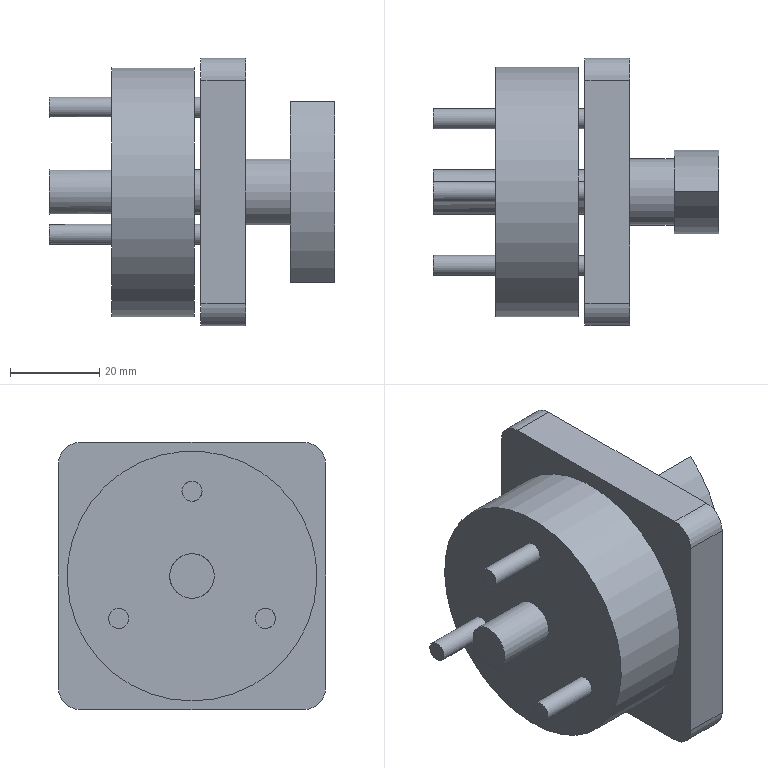Part | STEP file | 冲床-300配套压波_id418_x_t | 1 solid | 30 faces | box 64 x 60 x 60 mm | volume 90346 mm3 | cylinder 16 | plane 14 | commonest cylinder face diameters 4.5 x6 10 x6 53.607 x2 15 x1 56 x1
STEP:
#1=CARTESIAN_POINT('',(1921.2,181.454,-152.25));
#2=VERTEX_POINT('',#1);
#3=CARTESIAN_POINT('',(1921.2,181.454,-154.5));
#4=DIRECTION('',(1.,0.,0.));
#5=DIRECTION('',(0.,0.,1.));
#6=AXIS2_PLACEMENT_3D('',#3,#4,#5);
#7=CIRCLE('',#6,2.25);
#8=EDGE_CURVE('',#2,#2,#7,.T.);
#9=ORIENTED_EDGE('',*,*,#8,.F.);
#10=EDGE_LOOP('',(#9));
#11=FACE_BOUND('',#10,.T.);
#12=CARTESIAN_POINT('',(1919.7,181.454,-156.75));
#13=VERTEX_POINT('',#12);
#14=CARTESIAN_POINT('',(1919.7,181.454,-154.5));
#15=DIRECTION('',(1.,0.,0.));
#16=DIRECTION('',(0.,0.,-1.));
#17=AXIS2_PLACEMENT_3D('',#14,#15,#16);
#18=CIRCLE('',#17,2.25);
#19=EDGE_CURVE('',#13,#13,#18,.T.);
#20=ORIENTED_EDGE('',*,*,#19,.T.);
#21=EDGE_LOOP('',(#20));
#22=FACE_BOUND('',#21,.T.);
#23=CARTESIAN_POINT('',(1887.2,181.454,-154.5));
#24=DIRECTION('',(1.,0.,0.));
#25=DIRECTION('',(0.,0.,1.));
#26=AXIS2_PLACEMENT_3D('',#23,#24,#25);
#27=CYLINDRICAL_SURFACE('',#26,2.25);
#28=ADVANCED_FACE('',(#11,#22),#27,.T.);
#29=CARTESIAN_POINT('',(1921.2,165.,-123.75));
#30=VERTEX_POINT('',#29);
#31=CARTESIAN_POINT('',(1921.2,165.,-126.));
#32=DIRECTION('',(1.,0.,0.));
#33=DIRECTION('',(0.,0.,1.));
#34=AXIS2_PLACEMENT_3D('',#31,#32,#33);
#35=CIRCLE('',#34,2.25);
#36=EDGE_CURVE('',#30,#30,#35,.T.);
#37=ORIENTED_EDGE('',*,*,#36,.F.);
#38=EDGE_LOOP('',(#37));
#39=FACE_BOUND('',#38,.T.);
#40=CARTESIAN_POINT('',(1919.7,165.,-128.25));
#41=VERTEX_POINT('',#40);
#42=CARTESIAN_POINT('',(1919.7,165.,-126.));
#43=DIRECTION('',(1.,0.,0.));
#44=DIRECTION('',(0.,0.,-1.));
#45=AXIS2_PLACEMENT_3D('',#42,#43,#44);
#46=CIRCLE('',#45,2.25);
#47=EDGE_CURVE('',#41,#41,#46,.T.);
#48=ORIENTED_EDGE('',*,*,#47,.T.);
#49=EDGE_LOOP('',(#48));
#50=FACE_BOUND('',#49,.T.);
#51=CARTESIAN_POINT('',(1887.2,165.,-126.));
#52=DIRECTION('',(1.,0.,0.));
#53=DIRECTION('',(0.,0.,1.));
#54=AXIS2_PLACEMENT_3D('',#51,#52,#53);
#55=CYLINDRICAL_SURFACE('',#54,2.25);
#56=ADVANCED_FACE('',(#39,#50),#55,.T.);
#57=CARTESIAN_POINT('',(1921.2,165.,-140.));
#58=VERTEX_POINT('',#57);
#59=CARTESIAN_POINT('',(1921.2,165.,-145.));
#60=DIRECTION('',(1.,0.,0.));
#61=DIRECTION('',(0.,0.,1.));
#62=AXIS2_PLACEMENT_3D('',#59,#60,#61);
#63=CIRCLE('',#62,5.);
#64=EDGE_CURVE('',#58,#58,#63,.T.);
#65=ORIENTED_EDGE('',*,*,#64,.F.);
#66=EDGE_LOOP('',(#65));
#67=FACE_BOUND('',#66,.T.);
#68=CARTESIAN_POINT('',(1919.7,165.,-150.));
#69=VERTEX_POINT('',#68);
#70=CARTESIAN_POINT('',(1919.7,165.,-145.));
#71=DIRECTION('',(1.,0.,0.));
#72=DIRECTION('',(0.,0.,-1.));
#73=AXIS2_PLACEMENT_3D('',#70,#71,#72);
#74=CIRCLE('',#73,5.);
#75=EDGE_CURVE('',#69,#69,#74,.T.);
#76=ORIENTED_EDGE('',*,*,#75,.T.);
#77=EDGE_LOOP('',(#76));
#78=FACE_BOUND('',#77,.T.);
#79=CARTESIAN_POINT('',(1887.2,165.,-145.));
#80=DIRECTION('',(1.,0.,0.));
#81=DIRECTION('',(0.,0.,1.));
#82=AXIS2_PLACEMENT_3D('',#79,#80,#81);
#83=CYLINDRICAL_SURFACE('',#82,5.);
#84=ADVANCED_FACE('',(#67,#78),#83,.T.);
#85=CARTESIAN_POINT('',(1921.2,148.546,-152.25));
#86=VERTEX_POINT('',#85);
#87=CARTESIAN_POINT('',(1921.2,148.546,-154.5));
#88=DIRECTION('',(1.,0.,0.));
#89=DIRECTION('',(0.,0.,1.));
#90=AXIS2_PLACEMENT_3D('',#87,#88,#89);
#91=CIRCLE('',#90,2.25);
#92=EDGE_CURVE('',#86,#86,#91,.T.);
#93=ORIENTED_EDGE('',*,*,#92,.F.);
#94=EDGE_LOOP('',(#93));
#95=FACE_BOUND('',#94,.T.);
#96=CARTESIAN_POINT('',(1919.7,148.546,-156.75));
#97=VERTEX_POINT('',#96);
#98=CARTESIAN_POINT('',(1919.7,148.546,-154.5));
#99=DIRECTION('',(1.,0.,0.));
#100=DIRECTION('',(0.,0.,-1.));
#101=AXIS2_PLACEMENT_3D('',#98,#99,#100);
#102=CIRCLE('',#101,2.25);
#103=EDGE_CURVE('',#97,#97,#102,.T.);
#104=ORIENTED_EDGE('',*,*,#103,.T.);
#105=EDGE_LOOP('',(#104));
#106=FACE_BOUND('',#105,.T.);
#107=CARTESIAN_POINT('',(1887.2,148.546,-154.5));
#108=DIRECTION('',(1.,0.,0.));
#109=DIRECTION('',(0.,0.,1.));
#110=AXIS2_PLACEMENT_3D('',#107,#108,#109);
#111=CYLINDRICAL_SURFACE('',#110,2.25);
#112=ADVANCED_FACE('',(#95,#106),#111,.T.);
#113=CARTESIAN_POINT('',(1931.2,135.,-120.));
#114=VERTEX_POINT('',#113);
#115=CARTESIAN_POINT('',(1931.2,135.,-170.));
#116=VERTEX_POINT('',#115);
#117=CARTESIAN_POINT('',(1931.2,135.,-175.));
#118=DIRECTION('',(0.,0.,-1.));
#119=VECTOR('',#118,1.);
#120=LINE('',#117,#119);
#121=EDGE_CURVE('',#114,#116,#120,.T.);
#122=ORIENTED_EDGE('',*,*,#121,.F.);
#123=CARTESIAN_POINT('',(1921.2,135.,-120.));
#124=VERTEX_POINT('',#123);
#125=CARTESIAN_POINT('',(1931.2,135.,-120.));
#126=DIRECTION('',(-1.,0.,0.));
#127=VECTOR('',#126,1.);
#128=LINE('',#125,#127);
#129=EDGE_CURVE('',#114,#124,#128,.T.);
#130=ORIENTED_EDGE('',*,*,#129,.T.);
#131=CARTESIAN_POINT('',(1921.2,135.,-170.));
#132=VERTEX_POINT('',#131);
#133=CARTESIAN_POINT('',(1921.2,135.,-175.));
#134=DIRECTION('',(0.,0.,-1.));
#135=VECTOR('',#134,1.);
#136=LINE('',#133,#135);
#137=EDGE_CURVE('',#124,#132,#136,.T.);
#138=ORIENTED_EDGE('',*,*,#137,.T.);
#139=CARTESIAN_POINT('',(1931.2,135.,-170.));
#140=DIRECTION('',(1.,0.,0.));
#141=VECTOR('',#140,1.);
#142=LINE('',#139,#141);
#143=EDGE_CURVE('',#132,#116,#142,.T.);
#144=ORIENTED_EDGE('',*,*,#143,.T.);
#145=EDGE_LOOP('',(#122,#130,#138,#144));
#146=FACE_OUTER_BOUND('',#145,.T.);
#147=CARTESIAN_POINT('',(1931.2,135.,-175.));
#148=DIRECTION('',(0.,1.,0.));
#149=DIRECTION('',(0.,0.,-1.));
#150=AXIS2_PLACEMENT_3D('',#147,#148,#149);
#151=PLANE('',#150);
#152=ADVANCED_FACE('',(#146),#151,.F.);
#153=CARTESIAN_POINT('',(1921.2,190.,-115.));
#154=VERTEX_POINT('',#153);
#155=CARTESIAN_POINT('',(1921.2,140.,-115.));
#156=VERTEX_POINT('',#155);
#157=CARTESIAN_POINT('',(1921.2,135.,-115.));
#158=DIRECTION('',(0.,-1.,0.));
#159=VECTOR('',#158,1.);
#160=LINE('',#157,#159);
#161=EDGE_CURVE('',#154,#156,#160,.T.);
#162=ORIENTED_EDGE('',*,*,#161,.T.);
#163=CARTESIAN_POINT('',(1931.2,140.,-115.));
#164=VERTEX_POINT('',#163);
#165=CARTESIAN_POINT('',(1931.2,140.,-115.));
#166=DIRECTION('',(1.,0.,0.));
#167=VECTOR('',#166,1.);
#168=LINE('',#165,#167);
#169=EDGE_CURVE('',#156,#164,#168,.T.);
#170=ORIENTED_EDGE('',*,*,#169,.T.);
#171=CARTESIAN_POINT('',(1931.2,190.,-115.));
#172=VERTEX_POINT('',#171);
#173=CARTESIAN_POINT('',(1931.2,135.,-115.));
#174=DIRECTION('',(0.,-1.,0.));
#175=VECTOR('',#174,1.);
#176=LINE('',#173,#175);
#177=EDGE_CURVE('',#172,#164,#176,.T.);
#178=ORIENTED_EDGE('',*,*,#177,.F.);
#179=CARTESIAN_POINT('',(1931.2,190.,-115.));
#180=DIRECTION('',(-1.,0.,0.));
#181=VECTOR('',#180,1.);
#182=LINE('',#179,#181);
#183=EDGE_CURVE('',#172,#154,#182,.T.);
#184=ORIENTED_EDGE('',*,*,#183,.T.);
#185=EDGE_LOOP('',(#162,#170,#178,#184));
#186=FACE_OUTER_BOUND('',#185,.T.);
#187=CARTESIAN_POINT('',(1931.2,135.,-115.));
#188=DIRECTION('',(0.,0.,-1.));
#189=DIRECTION('',(0.,-1.,0.));
#190=AXIS2_PLACEMENT_3D('',#187,#188,#189);
#191=PLANE('',#190);
#192=ADVANCED_FACE('',(#186),#191,.F.);
#193=CARTESIAN_POINT('',(1921.2,195.,-170.));
#194=VERTEX_POINT('',#193);
#195=CARTESIAN_POINT('',(1921.2,195.,-120.));
#196=VERTEX_POINT('',#195);
#197=CARTESIAN_POINT('',(1921.2,195.,-115.));
#198=DIRECTION('',(0.,0.,1.));
#199=VECTOR('',#198,1.);
#200=LINE('',#197,#199);
#201=EDGE_CURVE('',#194,#196,#200,.T.);
#202=ORIENTED_EDGE('',*,*,#201,.T.);
#203=CARTESIAN_POINT('',(1931.2,195.,-120.));
#204=VERTEX_POINT('',#203);
#205=CARTESIAN_POINT('',(1931.2,195.,-120.));
#206=DIRECTION('',(1.,0.,0.));
#207=VECTOR('',#206,1.);
#208=LINE('',#205,#207);
#209=EDGE_CURVE('',#196,#204,#208,.T.);
#210=ORIENTED_EDGE('',*,*,#209,.T.);
#211=CARTESIAN_POINT('',(1931.2,195.,-170.));
#212=VERTEX_POINT('',#211);
#213=CARTESIAN_POINT('',(1931.2,195.,-115.));
#214=DIRECTION('',(0.,0.,1.));
#215=VECTOR('',#214,1.);
#216=LINE('',#213,#215);
#217=EDGE_CURVE('',#212,#204,#216,.T.);
#218=ORIENTED_EDGE('',*,*,#217,.F.);
#219=CARTESIAN_POINT('',(1931.2,195.,-170.));
#220=DIRECTION('',(-1.,0.,0.));
#221=VECTOR('',#220,1.);
#222=LINE('',#219,#221);
#223=EDGE_CURVE('',#212,#194,#222,.T.);
#224=ORIENTED_EDGE('',*,*,#223,.T.);
#225=EDGE_LOOP('',(#202,#210,#218,#224));
#226=FACE_OUTER_BOUND('',#225,.T.);
#227=CARTESIAN_POINT('',(1931.2,195.,-115.));
#228=DIRECTION('',(0.,-1.,0.));
#229=DIRECTION('',(0.,0.,1.));
#230=AXIS2_PLACEMENT_3D('',#227,#228,#229);
#231=PLANE('',#230);
#232=ADVANCED_FACE('',(#226),#231,.F.);
#233=CARTESIAN_POINT('',(1931.2,140.,-175.));
#234=VERTEX_POINT('',#233);
#235=CARTESIAN_POINT('',(1931.2,190.,-175.));
#236=VERTEX_POINT('',#235);
#237=CARTESIAN_POINT('',(1931.2,195.,-175.));
#238=DIRECTION('',(0.,1.,0.));
#239=VECTOR('',#238,1.);
#240=LINE('',#237,#239);
#241=EDGE_CURVE('',#234,#236,#240,.T.);
#242=ORIENTED_EDGE('',*,*,#241,.F.);
#243=CARTESIAN_POINT('',(1921.2,140.,-175.));
#244=VERTEX_POINT('',#243);
#245=CARTESIAN_POINT('',(1931.2,140.,-175.));
#246=DIRECTION('',(-1.,0.,0.));
#247=VECTOR('',#246,1.);
#248=LINE('',#245,#247);
#249=EDGE_CURVE('',#234,#244,#248,.T.);
#250=ORIENTED_EDGE('',*,*,#249,.T.);
#251=CARTESIAN_POINT('',(1921.2,190.,-175.));
#252=VERTEX_POINT('',#251);
#253=CARTESIAN_POINT('',(1921.2,195.,-175.));
#254=DIRECTION('',(0.,1.,0.));
#255=VECTOR('',#254,1.);
#256=LINE('',#253,#255);
#257=EDGE_CURVE('',#244,#252,#256,.T.);
#258=ORIENTED_EDGE('',*,*,#257,.T.);
#259=CARTESIAN_POINT('',(1931.2,190.,-175.));
#260=DIRECTION('',(1.,0.,0.));
#261=VECTOR('',#260,1.);
#262=LINE('',#259,#261);
#263=EDGE_CURVE('',#252,#236,#262,.T.);
#264=ORIENTED_EDGE('',*,*,#263,.T.);
#265=EDGE_LOOP('',(#242,#250,#258,#264));
#266=FACE_OUTER_BOUND('',#265,.T.);
#267=CARTESIAN_POINT('',(1931.2,195.,-175.));
#268=DIRECTION('',(0.,0.,1.));
#269=DIRECTION('',(0.,1.,0.));
#270=AXIS2_PLACEMENT_3D('',#267,#268,#269);
#271=PLANE('',#270);
#272=ADVANCED_FACE('',(#266),#271,.F.);
#273=CARTESIAN_POINT('',(1931.2,157.5,-145.));
#274=VERTEX_POINT('',#273);
#275=CARTESIAN_POINT('',(1931.2,165.,-145.));
#276=DIRECTION('',(-1.,0.,0.));
#277=DIRECTION('',(0.,-1.,0.));
#278=AXIS2_PLACEMENT_3D('',#275,#276,#277);
#279=CIRCLE('',#278,7.5);
#280=EDGE_CURVE('',#274,#274,#279,.T.);
#281=ORIENTED_EDGE('',*,*,#280,.T.);
#282=EDGE_LOOP('',(#281));
#283=FACE_BOUND('',#282,.T.);
#284=ORIENTED_EDGE('',*,*,#217,.T.);
#285=CARTESIAN_POINT('',(1931.2,190.,-120.));
#286=DIRECTION('',(1.,0.,0.));
#287=DIRECTION('',(0.,0.,1.));
#288=AXIS2_PLACEMENT_3D('',#285,#286,#287);
#289=CIRCLE('',#288,5.);
#290=EDGE_CURVE('',#204,#172,#289,.T.);
#291=ORIENTED_EDGE('',*,*,#290,.T.);
#292=ORIENTED_EDGE('',*,*,#177,.T.);
#293=CARTESIAN_POINT('',(1931.2,140.,-120.));
#294=DIRECTION('',(1.,0.,0.));
#295=DIRECTION('',(0.,0.,1.));
#296=AXIS2_PLACEMENT_3D('',#293,#294,#295);
#297=CIRCLE('',#296,5.);
#298=EDGE_CURVE('',#164,#114,#297,.T.);
#299=ORIENTED_EDGE('',*,*,#298,.T.);
#300=ORIENTED_EDGE('',*,*,#121,.T.);
#301=CARTESIAN_POINT('',(1931.2,140.,-170.));
#302=DIRECTION('',(1.,0.,0.));
#303=DIRECTION('',(0.,0.,1.));
#304=AXIS2_PLACEMENT_3D('',#301,#302,#303);
#305=CIRCLE('',#304,5.);
#306=EDGE_CURVE('',#116,#234,#305,.T.);
#307=ORIENTED_EDGE('',*,*,#306,.T.);
#308=ORIENTED_EDGE('',*,*,#241,.T.);
#309=CARTESIAN_POINT('',(1931.2,190.,-170.));
#310=DIRECTION('',(1.,0.,0.));
#311=DIRECTION('',(0.,0.,1.));
#312=AXIS2_PLACEMENT_3D('',#309,#310,#311);
#313=CIRCLE('',#312,5.);
#314=EDGE_CURVE('',#236,#212,#313,.T.);
#315=ORIENTED_EDGE('',*,*,#314,.T.);
#316=EDGE_LOOP('',(#284,#291,#292,#299,#300,#307,#308,#315));
#317=FACE_BOUND('',#316,.T.);
#318=CARTESIAN_POINT('',(1931.2,885.,370.));
#319=DIRECTION('',(1.,0.,0.));
#320=DIRECTION('',(0.,0.,1.));
#321=AXIS2_PLACEMENT_3D('',#318,#319,#320);
#322=PLANE('',#321);
#323=ADVANCED_FACE('',(#283,#317),#322,.T.);
#324=ORIENTED_EDGE('',*,*,#92,.T.);
#325=EDGE_LOOP('',(#324));
#326=FACE_BOUND('',#325,.T.);
#327=ORIENTED_EDGE('',*,*,#64,.T.);
#328=EDGE_LOOP('',(#327));
#329=FACE_BOUND('',#328,.T.);
#330=ORIENTED_EDGE('',*,*,#36,.T.);
#331=EDGE_LOOP('',(#330));
#332=FACE_BOUND('',#331,.T.);
#333=ORIENTED_EDGE('',*,*,#8,.T.);
#334=EDGE_LOOP('',(#333));
#335=FACE_BOUND('',#334,.T.);
#336=ORIENTED_EDGE('',*,*,#257,.F.);
#337=CARTESIAN_POINT('',(1921.2,140.,-170.));
#338=DIRECTION('',(-1.,0.,0.));
#339=DIRECTION('',(0.,0.,1.));
#340=AXIS2_PLACEMENT_3D('',#337,#338,#339);
#341=CIRCLE('',#340,5.);
#342=EDGE_CURVE('',#244,#132,#341,.T.);
#343=ORIENTED_EDGE('',*,*,#342,.T.);
#344=ORIENTED_EDGE('',*,*,#137,.F.);
#345=CARTESIAN_POINT('',(1921.2,140.,-120.));
#346=DIRECTION('',(-1.,0.,0.));
#347=DIRECTION('',(0.,0.,1.));
#348=AXIS2_PLACEMENT_3D('',#345,#346,#347);
#349=CIRCLE('',#348,5.);
#350=EDGE_CURVE('',#124,#156,#349,.T.);
#351=ORIENTED_EDGE('',*,*,#350,.T.);
#352=ORIENTED_EDGE('',*,*,#161,.F.);
#353=CARTESIAN_POINT('',(1921.2,190.,-120.));
#354=DIRECTION('',(-1.,0.,0.));
#355=DIRECTION('',(0.,0.,1.));
#356=AXIS2_PLACEMENT_3D('',#353,#354,#355);
#357=CIRCLE('',#356,5.);
#358=EDGE_CURVE('',#154,#196,#357,.T.);
#359=ORIENTED_EDGE('',*,*,#358,.T.);
#360=ORIENTED_EDGE('',*,*,#201,.F.);
#361=CARTESIAN_POINT('',(1921.2,190.,-170.));
#362=DIRECTION('',(-1.,0.,0.));
#363=DIRECTION('',(0.,0.,1.));
#364=AXIS2_PLACEMENT_3D('',#361,#362,#363);
#365=CIRCLE('',#364,5.);
#366=EDGE_CURVE('',#194,#252,#365,.T.);
#367=ORIENTED_EDGE('',*,*,#366,.T.);
#368=EDGE_LOOP('',(#336,#343,#344,#351,#352,#359,#360,#367));
#369=FACE_BOUND('',#368,.T.);
#370=CARTESIAN_POINT('',(1921.2,885.,370.));
#371=DIRECTION('',(1.,0.,0.));
#372=DIRECTION('',(0.,0.,1.));
#373=AXIS2_PLACEMENT_3D('',#370,#371,#372);
#374=PLANE('',#373);
#375=ADVANCED_FACE('',(#326,#329,#332,#335,#369),#374,.F.);
#376=CARTESIAN_POINT('',(1941.2,157.5,-145.));
#377=VERTEX_POINT('',#376);
#378=CARTESIAN_POINT('',(1941.2,165.,-145.));
#379=DIRECTION('',(-1.,0.,0.));
#380=DIRECTION('',(0.,-1.,0.));
#381=AXIS2_PLACEMENT_3D('',#378,#379,#380);
#382=CIRCLE('',#381,7.5);
#383=EDGE_CURVE('',#377,#377,#382,.T.);
#384=ORIENTED_EDGE('',*,*,#383,.T.);
#385=EDGE_LOOP('',(#384));
#386=FACE_BOUND('',#385,.T.);
#387=ORIENTED_EDGE('',*,*,#280,.F.);
#388=EDGE_LOOP('',(#387));
#389=FACE_BOUND('',#388,.T.);
#390=CARTESIAN_POINT('',(1941.2,165.,-145.));
#391=DIRECTION('',(-1.,0.,0.));
#392=DIRECTION('',(0.,0.,-1.));
#393=AXIS2_PLACEMENT_3D('',#390,#391,#392);
#394=CYLINDRICAL_SURFACE('',#393,7.5);
#395=ADVANCED_FACE('',(#386,#389),#394,.T.);
#396=CARTESIAN_POINT('',(1941.2,165.,-124.667));
#397=VERTEX_POINT('',#396);
#398=CARTESIAN_POINT('',(1941.2,165.,-165.333));
#399=VERTEX_POINT('',#398);
#400=CARTESIAN_POINT('',(1941.2,182.465,-145.));
#401=DIRECTION('',(1.,0.,0.));
#402=DIRECTION('',(0.,1.,0.));
#403=AXIS2_PLACEMENT_3D('',#400,#401,#402);
#404=CIRCLE('',#403,26.804);
#405=EDGE_CURVE('',#397,#399,#404,.T.);
#406=ORIENTED_EDGE('',*,*,#405,.T.);
#407=CARTESIAN_POINT('',(1951.2,165.,-165.333));
#408=VERTEX_POINT('',#407);
#409=CARTESIAN_POINT('',(1951.2,165.,-165.333));
#410=DIRECTION('',(-1.,0.,0.));
#411=VECTOR('',#410,1.);
#412=LINE('',#409,#411);
#413=EDGE_CURVE('',#408,#399,#412,.T.);
#414=ORIENTED_EDGE('',*,*,#413,.F.);
#415=CARTESIAN_POINT('',(1951.2,165.,-124.667));
#416=VERTEX_POINT('',#415);
#417=CARTESIAN_POINT('',(1951.2,182.465,-145.));
#418=DIRECTION('',(1.,0.,0.));
#419=DIRECTION('',(0.,1.,0.));
#420=AXIS2_PLACEMENT_3D('',#417,#418,#419);
#421=CIRCLE('',#420,26.804);
#422=EDGE_CURVE('',#416,#408,#421,.T.);
#423=ORIENTED_EDGE('',*,*,#422,.F.);
#424=CARTESIAN_POINT('',(1951.2,165.,-124.667));
#425=DIRECTION('',(1.,0.,0.));
#426=VECTOR('',#425,1.);
#427=LINE('',#424,#426);
#428=EDGE_CURVE('',#397,#416,#427,.T.);
#429=ORIENTED_EDGE('',*,*,#428,.F.);
#430=EDGE_LOOP('',(#406,#414,#423,#429));
#431=FACE_OUTER_BOUND('',#430,.T.);
#432=CARTESIAN_POINT('',(1951.2,182.465,-145.));
#433=DIRECTION('',(-1.,0.,0.));
#434=DIRECTION('',(0.,0.,-1.));
#435=AXIS2_PLACEMENT_3D('',#432,#433,#434);
#436=CYLINDRICAL_SURFACE('',#435,26.804);
#437=ADVANCED_FACE('',(#431),#436,.T.);
#438=CARTESIAN_POINT('',(1941.2,147.535,-145.));
#439=DIRECTION('',(1.,0.,0.));
#440=DIRECTION('',(0.,-1.,0.));
#441=AXIS2_PLACEMENT_3D('',#438,#439,#440);
#442=CIRCLE('',#441,26.804);
#443=EDGE_CURVE('',#399,#397,#442,.T.);
#444=ORIENTED_EDGE('',*,*,#443,.T.);
#445=ORIENTED_EDGE('',*,*,#428,.T.);
#446=CARTESIAN_POINT('',(1951.2,147.535,-145.));
#447=DIRECTION('',(1.,0.,0.));
#448=DIRECTION('',(0.,-1.,0.));
#449=AXIS2_PLACEMENT_3D('',#446,#447,#448);
#450=CIRCLE('',#449,26.804);
#451=EDGE_CURVE('',#408,#416,#450,.T.);
#452=ORIENTED_EDGE('',*,*,#451,.F.);
#453=ORIENTED_EDGE('',*,*,#413,.T.);
#454=EDGE_LOOP('',(#444,#445,#452,#453));
#455=FACE_OUTER_BOUND('',#454,.T.);
#456=CARTESIAN_POINT('',(1951.2,147.535,-145.));
#457=DIRECTION('',(-1.,0.,0.));
#458=DIRECTION('',(0.,0.,-1.));
#459=AXIS2_PLACEMENT_3D('',#456,#457,#458);
#460=CYLINDRICAL_SURFACE('',#459,26.804);
#461=ADVANCED_FACE('',(#455),#460,.T.);
#462=ORIENTED_EDGE('',*,*,#422,.T.);
#463=ORIENTED_EDGE('',*,*,#451,.T.);
#464=EDGE_LOOP('',(#462,#463));
#465=FACE_OUTER_BOUND('',#464,.T.);
#466=CARTESIAN_POINT('',(1951.2,165.,-145.));
#467=DIRECTION('',(1.,0.,0.));
#468=DIRECTION('',(0.,0.,1.));
#469=AXIS2_PLACEMENT_3D('',#466,#467,#468);
#470=PLANE('',#469);
#471=ADVANCED_FACE('',(#465),#470,.T.);
#472=ORIENTED_EDGE('',*,*,#383,.F.);
#473=EDGE_LOOP('',(#472));
#474=FACE_BOUND('',#473,.T.);
#475=ORIENTED_EDGE('',*,*,#405,.F.);
#476=ORIENTED_EDGE('',*,*,#443,.F.);
#477=EDGE_LOOP('',(#475,#476));
#478=FACE_BOUND('',#477,.T.);
#479=CARTESIAN_POINT('',(1941.2,165.,-145.));
#480=DIRECTION('',(1.,0.,0.));
#481=DIRECTION('',(0.,0.,1.));
#482=AXIS2_PLACEMENT_3D('',#479,#480,#481);
#483=PLANE('',#482);
#484=ADVANCED_FACE('',(#474,#478),#483,.F.);
#485=ORIENTED_EDGE('',*,*,#314,.F.);
#486=ORIENTED_EDGE('',*,*,#263,.F.);
#487=ORIENTED_EDGE('',*,*,#366,.F.);
#488=ORIENTED_EDGE('',*,*,#223,.F.);
#489=EDGE_LOOP('',(#485,#486,#487,#488));
#490=FACE_OUTER_BOUND('',#489,.T.);
#491=CARTESIAN_POINT('',(1931.2,190.,-170.));
#492=DIRECTION('',(-1.,0.,0.));
#493=DIRECTION('',(0.,0.,-1.));
#494=AXIS2_PLACEMENT_3D('',#491,#492,#493);
#495=CYLINDRICAL_SURFACE('',#494,5.);
#496=ADVANCED_FACE('',(#490),#495,.T.);
#497=ORIENTED_EDGE('',*,*,#290,.F.);
#498=ORIENTED_EDGE('',*,*,#209,.F.);
#499=ORIENTED_EDGE('',*,*,#358,.F.);
#500=ORIENTED_EDGE('',*,*,#183,.F.);
#501=EDGE_LOOP('',(#497,#498,#499,#500));
#502=FACE_OUTER_BOUND('',#501,.T.);
#503=CARTESIAN_POINT('',(1931.2,190.,-120.));
#504=DIRECTION('',(-1.,0.,0.));
#505=DIRECTION('',(0.,0.,-1.));
#506=AXIS2_PLACEMENT_3D('',#503,#504,#505);
#507=CYLINDRICAL_SURFACE('',#506,5.);
#508=ADVANCED_FACE('',(#502),#507,.T.);
#509=ORIENTED_EDGE('',*,*,#306,.F.);
#510=ORIENTED_EDGE('',*,*,#143,.F.);
#511=ORIENTED_EDGE('',*,*,#342,.F.);
#512=ORIENTED_EDGE('',*,*,#249,.F.);
#513=EDGE_LOOP('',(#509,#510,#511,#512));
#514=FACE_OUTER_BOUND('',#513,.T.);
#515=CARTESIAN_POINT('',(1931.2,140.,-170.));
#516=DIRECTION('',(-1.,0.,0.));
#517=DIRECTION('',(0.,0.,-1.));
#518=AXIS2_PLACEMENT_3D('',#515,#516,#517);
#519=CYLINDRICAL_SURFACE('',#518,5.);
#520=ADVANCED_FACE('',(#514),#519,.T.);
#521=ORIENTED_EDGE('',*,*,#298,.F.);
#522=ORIENTED_EDGE('',*,*,#169,.F.);
#523=ORIENTED_EDGE('',*,*,#350,.F.);
#524=ORIENTED_EDGE('',*,*,#129,.F.);
#525=EDGE_LOOP('',(#521,#522,#523,#524));
#526=FACE_OUTER_BOUND('',#525,.T.);
#527=CARTESIAN_POINT('',(1931.2,140.,-120.));
#528=DIRECTION('',(-1.,0.,0.));
#529=DIRECTION('',(0.,0.,-1.));
#530=AXIS2_PLACEMENT_3D('',#527,#528,#529);
#531=CYLINDRICAL_SURFACE('',#530,5.);
#532=ADVANCED_FACE('',(#526),#531,.T.);
#533=CARTESIAN_POINT('',(1901.2,165.,-173.));
#534=VERTEX_POINT('',#533);
#535=CARTESIAN_POINT('',(1901.2,165.,-145.));
#536=DIRECTION('',(-1.,0.,0.));
#537=DIRECTION('',(0.,0.,-1.));
#538=AXIS2_PLACEMENT_3D('',#535,#536,#537);
#539=CIRCLE('',#538,28.);
#540=EDGE_CURVE('',#534,#534,#539,.T.);
#541=ORIENTED_EDGE('',*,*,#540,.F.);
#542=EDGE_LOOP('',(#541));
#543=FACE_BOUND('',#542,.T.);
#544=CARTESIAN_POINT('',(1919.7,165.,-173.));
#545=VERTEX_POINT('',#544);
#546=CARTESIAN_POINT('',(1919.7,165.,-145.));
#547=DIRECTION('',(-1.,0.,0.));
#548=DIRECTION('',(0.,0.,-1.));
#549=AXIS2_PLACEMENT_3D('',#546,#547,#548);
#550=CIRCLE('',#549,28.);
#551=EDGE_CURVE('',#545,#545,#550,.T.);
#552=ORIENTED_EDGE('',*,*,#551,.T.);
#553=EDGE_LOOP('',(#552));
#554=FACE_BOUND('',#553,.T.);
#555=CARTESIAN_POINT('',(1901.2,165.,-145.));
#556=DIRECTION('',(1.,0.,0.));
#557=DIRECTION('',(0.,0.,1.));
#558=AXIS2_PLACEMENT_3D('',#555,#556,#557);
#559=CYLINDRICAL_SURFACE('',#558,28.);
#560=ADVANCED_FACE('',(#543,#554),#559,.T.);
#561=CARTESIAN_POINT('',(1901.2,181.454,-156.75));
#562=VERTEX_POINT('',#561);
#563=CARTESIAN_POINT('',(1901.2,181.454,-154.5));
#564=DIRECTION('',(1.,0.,0.));
#565=DIRECTION('',(0.,0.,-1.));
#566=AXIS2_PLACEMENT_3D('',#563,#564,#565);
#567=CIRCLE('',#566,2.25);
#568=EDGE_CURVE('',#562,#562,#567,.T.);
#569=ORIENTED_EDGE('',*,*,#568,.T.);
#570=EDGE_LOOP('',(#569));
#571=FACE_BOUND('',#570,.T.);
#572=CARTESIAN_POINT('',(1901.2,165.,-128.25));
#573=VERTEX_POINT('',#572);
#574=CARTESIAN_POINT('',(1901.2,165.,-126.));
#575=DIRECTION('',(1.,0.,0.));
#576=DIRECTION('',(0.,0.,-1.));
#577=AXIS2_PLACEMENT_3D('',#574,#575,#576);
#578=CIRCLE('',#577,2.25);
#579=EDGE_CURVE('',#573,#573,#578,.T.);
#580=ORIENTED_EDGE('',*,*,#579,.T.);
#581=EDGE_LOOP('',(#580));
#582=FACE_BOUND('',#581,.T.);
#583=CARTESIAN_POINT('',(1901.2,165.,-150.));
#584=VERTEX_POINT('',#583);
#585=CARTESIAN_POINT('',(1901.2,165.,-145.));
#586=DIRECTION('',(1.,0.,0.));
#587=DIRECTION('',(0.,0.,-1.));
#588=AXIS2_PLACEMENT_3D('',#585,#586,#587);
#589=CIRCLE('',#588,5.);
#590=EDGE_CURVE('',#584,#584,#589,.T.);
#591=ORIENTED_EDGE('',*,*,#590,.T.);
#592=EDGE_LOOP('',(#591));
#593=FACE_BOUND('',#592,.T.);
#594=CARTESIAN_POINT('',(1901.2,148.546,-156.75));
#595=VERTEX_POINT('',#594);
#596=CARTESIAN_POINT('',(1901.2,148.546,-154.5));
#597=DIRECTION('',(1.,0.,0.));
#598=DIRECTION('',(0.,0.,-1.));
#599=AXIS2_PLACEMENT_3D('',#596,#597,#598);
#600=CIRCLE('',#599,2.25);
#601=EDGE_CURVE('',#595,#595,#600,.T.);
#602=ORIENTED_EDGE('',*,*,#601,.T.);
#603=EDGE_LOOP('',(#602));
#604=FACE_BOUND('',#603,.T.);
#605=ORIENTED_EDGE('',*,*,#540,.T.);
#606=EDGE_LOOP('',(#605));
#607=FACE_BOUND('',#606,.T.);
#608=CARTESIAN_POINT('',(1901.2,165.,-145.));
#609=DIRECTION('',(-1.,0.,0.));
#610=DIRECTION('',(0.,0.,-1.));
#611=AXIS2_PLACEMENT_3D('',#608,#609,#610);
#612=PLANE('',#611);
#613=ADVANCED_FACE('',(#571,#582,#593,#604,#607),#612,.T.);
#614=ORIENTED_EDGE('',*,*,#19,.F.);
#615=EDGE_LOOP('',(#614));
#616=FACE_BOUND('',#615,.T.);
#617=ORIENTED_EDGE('',*,*,#47,.F.);
#618=EDGE_LOOP('',(#617));
#619=FACE_BOUND('',#618,.T.);
#620=ORIENTED_EDGE('',*,*,#75,.F.);
#621=EDGE_LOOP('',(#620));
#622=FACE_BOUND('',#621,.T.);
#623=ORIENTED_EDGE('',*,*,#103,.F.);
#624=EDGE_LOOP('',(#623));
#625=FACE_BOUND('',#624,.T.);
#626=ORIENTED_EDGE('',*,*,#551,.F.);
#627=EDGE_LOOP('',(#626));
#628=FACE_BOUND('',#627,.T.);
#629=CARTESIAN_POINT('',(1919.7,165.,-145.));
#630=DIRECTION('',(-1.,0.,0.));
#631=DIRECTION('',(0.,0.,-1.));
#632=AXIS2_PLACEMENT_3D('',#629,#630,#631);
#633=PLANE('',#632);
#634=ADVANCED_FACE('',(#616,#619,#622,#625,#628),#633,.F.);
#635=CARTESIAN_POINT('',(1887.2,149.671,-156.449));
#636=VERTEX_POINT('',#635);
#637=CARTESIAN_POINT('',(1887.2,148.546,-154.5));
#638=DIRECTION('',(1.,0.,0.));
#639=DIRECTION('',(0.,0.5,-0.866));
#640=AXIS2_PLACEMENT_3D('',#637,#638,#639);
#641=CIRCLE('',#640,2.25);
#642=EDGE_CURVE('',#636,#636,#641,.T.);
#643=ORIENTED_EDGE('',*,*,#642,.F.);
#644=EDGE_LOOP('',(#643));
#645=FACE_OUTER_BOUND('',#644,.T.);
#646=CARTESIAN_POINT('',(1887.2,148.546,-154.5));
#647=DIRECTION('',(1.,0.,0.));
#648=DIRECTION('',(0.,0.,1.));
#649=AXIS2_PLACEMENT_3D('',#646,#647,#648);
#650=PLANE('',#649);
#651=ADVANCED_FACE('',(#645),#650,.F.);
#652=ORIENTED_EDGE('',*,*,#601,.F.);
#653=EDGE_LOOP('',(#652));
#654=FACE_BOUND('',#653,.T.);
#655=ORIENTED_EDGE('',*,*,#642,.T.);
#656=EDGE_LOOP('',(#655));
#657=FACE_BOUND('',#656,.T.);
#658=CARTESIAN_POINT('',(1887.2,148.546,-154.5));
#659=DIRECTION('',(1.,0.,0.));
#660=DIRECTION('',(0.,0.,1.));
#661=AXIS2_PLACEMENT_3D('',#658,#659,#660);
#662=CYLINDRICAL_SURFACE('',#661,2.25);
#663=ADVANCED_FACE('',(#654,#657),#662,.T.);
#664=CARTESIAN_POINT('',(1887.2,160.,-145.));
#665=VERTEX_POINT('',#664);
#666=CARTESIAN_POINT('',(1887.2,165.,-145.));
#667=DIRECTION('',(1.,0.,0.));
#668=DIRECTION('',(0.,-1.,0.));
#669=AXIS2_PLACEMENT_3D('',#666,#667,#668);
#670=CIRCLE('',#669,5.);
#671=EDGE_CURVE('',#665,#665,#670,.T.);
#672=ORIENTED_EDGE('',*,*,#671,.F.);
#673=EDGE_LOOP('',(#672));
#674=FACE_OUTER_BOUND('',#673,.T.);
#675=CARTESIAN_POINT('',(1887.2,165.,-145.));
#676=DIRECTION('',(1.,0.,0.));
#677=DIRECTION('',(0.,0.,1.));
#678=AXIS2_PLACEMENT_3D('',#675,#676,#677);
#679=PLANE('',#678);
#680=ADVANCED_FACE('',(#674),#679,.F.);
#681=ORIENTED_EDGE('',*,*,#590,.F.);
#682=EDGE_LOOP('',(#681));
#683=FACE_BOUND('',#682,.T.);
#684=ORIENTED_EDGE('',*,*,#671,.T.);
#685=EDGE_LOOP('',(#684));
#686=FACE_BOUND('',#685,.T.);
#687=CARTESIAN_POINT('',(1887.2,165.,-145.));
#688=DIRECTION('',(1.,0.,0.));
#689=DIRECTION('',(0.,0.,1.));
#690=AXIS2_PLACEMENT_3D('',#687,#688,#689);
#691=CYLINDRICAL_SURFACE('',#690,5.);
#692=ADVANCED_FACE('',(#683,#686),#691,.T.);
#693=CARTESIAN_POINT('',(1887.2,162.75,-126.));
#694=VERTEX_POINT('',#693);
#695=CARTESIAN_POINT('',(1887.2,165.,-126.));
#696=DIRECTION('',(1.,0.,0.));
#697=DIRECTION('',(0.,-1.,0.));
#698=AXIS2_PLACEMENT_3D('',#695,#696,#697);
#699=CIRCLE('',#698,2.25);
#700=EDGE_CURVE('',#694,#694,#699,.T.);
#701=ORIENTED_EDGE('',*,*,#700,.F.);
#702=EDGE_LOOP('',(#701));
#703=FACE_OUTER_BOUND('',#702,.T.);
#704=CARTESIAN_POINT('',(1887.2,165.,-126.));
#705=DIRECTION('',(1.,0.,0.));
#706=DIRECTION('',(0.,0.,1.));
#707=AXIS2_PLACEMENT_3D('',#704,#705,#706);
#708=PLANE('',#707);
#709=ADVANCED_FACE('',(#703),#708,.F.);
#710=ORIENTED_EDGE('',*,*,#579,.F.);
#711=EDGE_LOOP('',(#710));
#712=FACE_BOUND('',#711,.T.);
#713=ORIENTED_EDGE('',*,*,#700,.T.);
#714=EDGE_LOOP('',(#713));
#715=FACE_BOUND('',#714,.T.);
#716=CARTESIAN_POINT('',(1887.2,165.,-126.));
#717=DIRECTION('',(1.,0.,0.));
#718=DIRECTION('',(0.,0.,1.));
#719=AXIS2_PLACEMENT_3D('',#716,#717,#718);
#720=CYLINDRICAL_SURFACE('',#719,2.25);
#721=ADVANCED_FACE('',(#712,#715),#720,.T.);
#722=CARTESIAN_POINT('',(1887.2,182.579,-152.551));
#723=VERTEX_POINT('',#722);
#724=CARTESIAN_POINT('',(1887.2,181.454,-154.5));
#725=DIRECTION('',(1.,0.,0.));
#726=DIRECTION('',(0.,0.5,0.866));
#727=AXIS2_PLACEMENT_3D('',#724,#725,#726);
#728=CIRCLE('',#727,2.25);
#729=EDGE_CURVE('',#723,#723,#728,.T.);
#730=ORIENTED_EDGE('',*,*,#729,.F.);
#731=EDGE_LOOP('',(#730));
#732=FACE_OUTER_BOUND('',#731,.T.);
#733=CARTESIAN_POINT('',(1887.2,181.454,-154.5));
#734=DIRECTION('',(1.,0.,0.));
#735=DIRECTION('',(0.,0.,1.));
#736=AXIS2_PLACEMENT_3D('',#733,#734,#735);
#737=PLANE('',#736);
#738=ADVANCED_FACE('',(#732),#737,.F.);
#739=ORIENTED_EDGE('',*,*,#568,.F.);
#740=EDGE_LOOP('',(#739));
#741=FACE_BOUND('',#740,.T.);
#742=ORIENTED_EDGE('',*,*,#729,.T.);
#743=EDGE_LOOP('',(#742));
#744=FACE_BOUND('',#743,.T.);
#745=CARTESIAN_POINT('',(1887.2,181.454,-154.5));
#746=DIRECTION('',(1.,0.,0.));
#747=DIRECTION('',(0.,0.,1.));
#748=AXIS2_PLACEMENT_3D('',#745,#746,#747);
#749=CYLINDRICAL_SURFACE('',#748,2.25);
#750=ADVANCED_FACE('',(#741,#744),#749,.T.);
#751=CLOSED_SHELL('',(#28,#56,#84,#112,#152,#192,#232,#272,#323,#375,#395,#437,#461,#471,#484,#496,#508,#520,#532,#560,#613,#634,#651,#663,#680,#692,#709,#721,#738,#750));
#752=MANIFOLD_SOLID_BREP('',#751);
#753=(LENGTH_UNIT()NAMED_UNIT(*)SI_UNIT(.MILLI.,.METRE.));
#754=UNCERTAINTY_MEASURE_WITH_UNIT(LENGTH_MEASURE(0.00002),#753,'','');
#755=(NAMED_UNIT(*)PLANE_ANGLE_UNIT()SI_UNIT($,.RADIAN.));
#756=PLANE_ANGLE_MEASURE_WITH_UNIT(PLANE_ANGLE_MEASURE(0.01745),#755);
#757=DIMENSIONAL_EXPONENTS(0.,0.,0.,0.,0.,0.,0.);
#758=(CONVERSION_BASED_UNIT('DEGREE',#756)NAMED_UNIT(#757)PLANE_ANGLE_UNIT());
#759=(NAMED_UNIT(*)SI_UNIT($,.STERADIAN.)SOLID_ANGLE_UNIT());
#760=(GEOMETRIC_REPRESENTATION_CONTEXT(3)GLOBAL_UNCERTAINTY_ASSIGNED_CONTEXT((#754))GLOBAL_UNIT_ASSIGNED_CONTEXT((#753,#758,#759))REPRESENTATION_CONTEXT('',''));
#761=ADVANCED_BREP_SHAPE_REPRESENTATION('',(#752),#760);